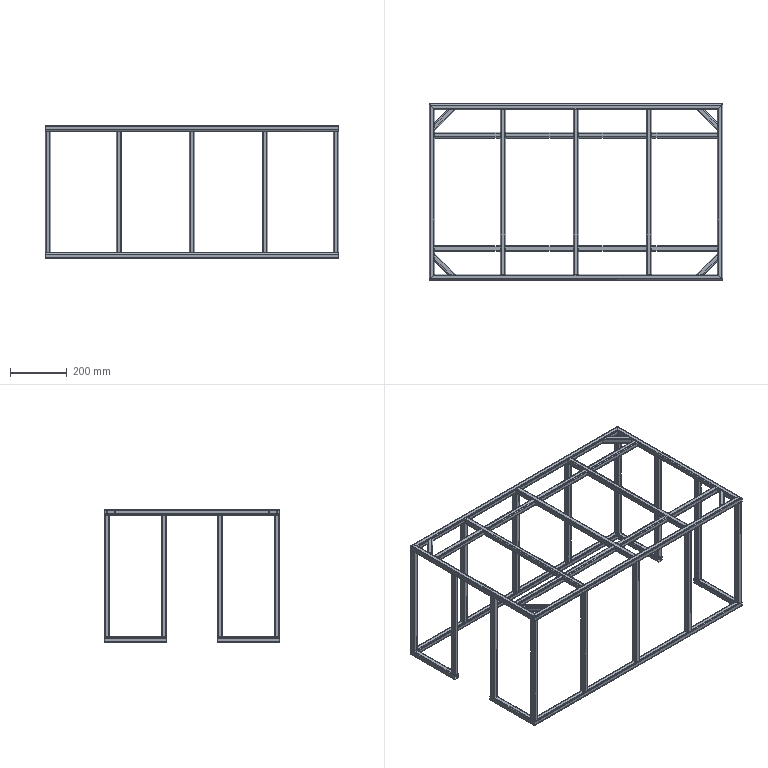Part | STEP file | KF-2212-070-001_Default<As Machined> | 39 solids | 710 faces | box 1036 x 620 x 470 mm | volume 2149735 mm3 | plane 390 | cylinder 320 | commonest cylinder face diameters 4 x156 8 x156 3.3 x8